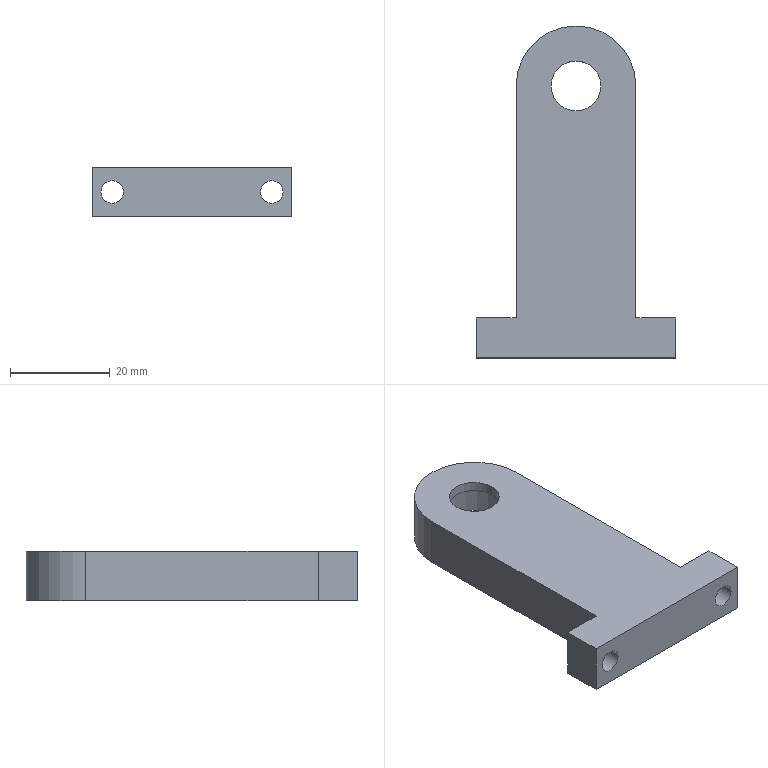Part | Creo | features CURVE 4, CUT 3, DATUM PLANE 3, COORDINATE SYSTEM 1, PROTRUSION 1 | 1 solid | 22 faces | box 40 x 66.5 x 10 mm | volume 14034 mm3 | plane 11 | cylinder 11 | commonest cylinder face diameters 4.5 x4 10 x2 15.636 x2 19 x2 24 x1
STEP:
#1=CARTESIAN_POINT('',(0.,0.,0.));
#2=DIRECTION('',(0.,0.,1.));
#3=DIRECTION('',(1.,0.,0.));
#4=AXIS2_PLACEMENT_3D('',#1,#2,#3);
#5=CARTESIAN_POINT('',(12.,54.5,0.));
#6=VERTEX_POINT('',#5);
#7=CARTESIAN_POINT('',(-12.,54.5,0.));
#8=VERTEX_POINT('',#7);
#9=CARTESIAN_POINT('',(0.,54.5,0.));
#10=DIRECTION('',(0.,0.,1.));
#11=DIRECTION('',(1.,0.,0.));
#12=AXIS2_PLACEMENT_3D('',#9,#10,#11);
#13=CIRCLE('',#12,12.);
#14=EDGE_CURVE('',#6,#8,#13,.T.);
#15=ORIENTED_EDGE('',*,*,#14,.T.);
#16=CARTESIAN_POINT('',(-12.,8.,0.));
#17=VERTEX_POINT('',#16);
#18=CARTESIAN_POINT('',(-12.,54.5,0.));
#19=DIRECTION('',(0.,-1.,0.));
#20=VECTOR('',#19,46.5);
#21=LINE('',#18,#20);
#22=EDGE_CURVE('',#8,#17,#21,.T.);
#23=ORIENTED_EDGE('',*,*,#22,.T.);
#24=CARTESIAN_POINT('',(-20.,8.,0.));
#25=VERTEX_POINT('',#24);
#26=CARTESIAN_POINT('',(-12.,8.,0.));
#27=DIRECTION('',(-1.,0.,0.));
#28=VECTOR('',#27,8.);
#29=LINE('',#26,#28);
#30=EDGE_CURVE('',#17,#25,#29,.T.);
#31=ORIENTED_EDGE('',*,*,#30,.T.);
#32=CARTESIAN_POINT('',(-20.,0.,0.));
#33=VERTEX_POINT('',#32);
#34=CARTESIAN_POINT('',(-20.,8.,0.));
#35=DIRECTION('',(0.,-1.,0.));
#36=VECTOR('',#35,8.);
#37=LINE('',#34,#36);
#38=EDGE_CURVE('',#25,#33,#37,.T.);
#39=ORIENTED_EDGE('',*,*,#38,.T.);
#40=CARTESIAN_POINT('',(20.,0.,0.));
#41=VERTEX_POINT('',#40);
#42=CARTESIAN_POINT('',(-20.,0.,0.));
#43=DIRECTION('',(1.,0.,0.));
#44=VECTOR('',#43,40.);
#45=LINE('',#42,#44);
#46=EDGE_CURVE('',#33,#41,#45,.T.);
#47=ORIENTED_EDGE('',*,*,#46,.T.);
#48=CARTESIAN_POINT('',(20.,8.,0.));
#49=VERTEX_POINT('',#48);
#50=CARTESIAN_POINT('',(20.,0.,0.));
#51=DIRECTION('',(0.,1.,0.));
#52=VECTOR('',#51,8.);
#53=LINE('',#50,#52);
#54=EDGE_CURVE('',#41,#49,#53,.T.);
#55=ORIENTED_EDGE('',*,*,#54,.T.);
#56=CARTESIAN_POINT('',(12.,8.,0.));
#57=VERTEX_POINT('',#56);
#58=CARTESIAN_POINT('',(20.,8.,0.));
#59=DIRECTION('',(-1.,0.,0.));
#60=VECTOR('',#59,8.);
#61=LINE('',#58,#60);
#62=EDGE_CURVE('',#49,#57,#61,.T.);
#63=ORIENTED_EDGE('',*,*,#62,.T.);
#64=CARTESIAN_POINT('',(12.,8.,0.));
#65=DIRECTION('',(0.,1.,0.));
#66=VECTOR('',#65,46.5);
#67=LINE('',#64,#66);
#68=EDGE_CURVE('',#57,#6,#67,.T.);
#69=ORIENTED_EDGE('',*,*,#68,.T.);
#70=EDGE_LOOP('',(#15,#23,#31,#39,#47,#55,#63,#69));
#71=FACE_OUTER_BOUND('',#70,.F.);
#72=CARTESIAN_POINT('',(-9.5,54.5,0.));
#73=VERTEX_POINT('',#72);
#74=CARTESIAN_POINT('',(9.5,54.5,0.));
#75=VERTEX_POINT('',#74);
#76=CARTESIAN_POINT('',(0.,54.5,0.));
#77=DIRECTION('',(0.,0.,-1.));
#78=DIRECTION('',(-1.,0.,0.));
#79=AXIS2_PLACEMENT_3D('',#76,#77,#78);
#80=CIRCLE('',#79,9.5);
#81=EDGE_CURVE('',#73,#75,#80,.T.);
#82=ORIENTED_EDGE('',*,*,#81,.T.);
#83=CARTESIAN_POINT('',(0.,54.5,0.));
#84=DIRECTION('',(0.,0.,-1.));
#85=DIRECTION('',(1.,0.,0.));
#86=AXIS2_PLACEMENT_3D('',#83,#84,#85);
#87=CIRCLE('',#86,9.5);
#88=EDGE_CURVE('',#75,#73,#87,.T.);
#89=ORIENTED_EDGE('',*,*,#88,.T.);
#90=EDGE_LOOP('',(#82,#89));
#91=FACE_BOUND('',#90,.F.);
#92=CARTESIAN_POINT('',(0.,0.,0.));
#93=DIRECTION('',(0.,0.,1.));
#94=DIRECTION('',(1.,0.,0.));
#95=AXIS2_PLACEMENT_3D('',#92,#93,#94);
#96=PLANE('',#95);
#97=ADVANCED_FACE('',(#71,#91),#96,.F.);
#98=ORIENTED_EDGE('',*,*,#14,.F.);
#99=CARTESIAN_POINT('',(12.,54.5,10.));
#100=VERTEX_POINT('',#99);
#101=CARTESIAN_POINT('',(12.,54.5,0.));
#102=DIRECTION('',(0.,0.,1.));
#103=VECTOR('',#102,10.);
#104=LINE('',#101,#103);
#105=EDGE_CURVE('',#6,#100,#104,.T.);
#106=ORIENTED_EDGE('',*,*,#105,.T.);
#107=CARTESIAN_POINT('',(-12.,54.5,10.));
#108=VERTEX_POINT('',#107);
#109=CARTESIAN_POINT('',(0.,54.5,10.));
#110=DIRECTION('',(0.,0.,1.));
#111=DIRECTION('',(1.,0.,0.));
#112=AXIS2_PLACEMENT_3D('',#109,#110,#111);
#113=CIRCLE('',#112,12.);
#114=EDGE_CURVE('',#100,#108,#113,.T.);
#115=ORIENTED_EDGE('',*,*,#114,.T.);
#116=CARTESIAN_POINT('',(-12.,54.5,0.));
#117=DIRECTION('',(0.,0.,1.));
#118=VECTOR('',#117,10.);
#119=LINE('',#116,#118);
#120=EDGE_CURVE('',#8,#108,#119,.T.);
#121=ORIENTED_EDGE('',*,*,#120,.F.);
#122=EDGE_LOOP('',(#98,#106,#115,#121));
#123=FACE_OUTER_BOUND('',#122,.F.);
#124=CARTESIAN_POINT('',(0.,54.5,0.));
#125=DIRECTION('',(0.,0.,1.));
#126=DIRECTION('',(1.,0.,0.));
#127=AXIS2_PLACEMENT_3D('',#124,#125,#126);
#128=CYLINDRICAL_SURFACE('',#127,12.);
#129=ADVANCED_FACE('',(#123),#128,.T.);
#130=ORIENTED_EDGE('',*,*,#68,.F.);
#131=CARTESIAN_POINT('',(12.,8.,10.));
#132=VERTEX_POINT('',#131);
#133=CARTESIAN_POINT('',(12.,8.,0.));
#134=DIRECTION('',(0.,0.,1.));
#135=VECTOR('',#134,10.);
#136=LINE('',#133,#135);
#137=EDGE_CURVE('',#57,#132,#136,.T.);
#138=ORIENTED_EDGE('',*,*,#137,.T.);
#139=CARTESIAN_POINT('',(12.,8.,10.));
#140=DIRECTION('',(0.,1.,0.));
#141=VECTOR('',#140,46.5);
#142=LINE('',#139,#141);
#143=EDGE_CURVE('',#132,#100,#142,.T.);
#144=ORIENTED_EDGE('',*,*,#143,.T.);
#145=ORIENTED_EDGE('',*,*,#105,.F.);
#146=EDGE_LOOP('',(#130,#138,#144,#145));
#147=FACE_OUTER_BOUND('',#146,.F.);
#148=CARTESIAN_POINT('',(12.,8.,0.));
#149=DIRECTION('',(1.,0.,0.));
#150=DIRECTION('',(0.,1.,0.));
#151=AXIS2_PLACEMENT_3D('',#148,#149,#150);
#152=PLANE('',#151);
#153=ADVANCED_FACE('',(#147),#152,.T.);
#154=ORIENTED_EDGE('',*,*,#62,.F.);
#155=CARTESIAN_POINT('',(20.,8.,10.));
#156=VERTEX_POINT('',#155);
#157=CARTESIAN_POINT('',(20.,8.,0.));
#158=DIRECTION('',(0.,0.,1.));
#159=VECTOR('',#158,10.);
#160=LINE('',#157,#159);
#161=EDGE_CURVE('',#49,#156,#160,.T.);
#162=ORIENTED_EDGE('',*,*,#161,.T.);
#163=CARTESIAN_POINT('',(20.,8.,10.));
#164=DIRECTION('',(-1.,0.,0.));
#165=VECTOR('',#164,8.);
#166=LINE('',#163,#165);
#167=EDGE_CURVE('',#156,#132,#166,.T.);
#168=ORIENTED_EDGE('',*,*,#167,.T.);
#169=ORIENTED_EDGE('',*,*,#137,.F.);
#170=EDGE_LOOP('',(#154,#162,#168,#169));
#171=FACE_OUTER_BOUND('',#170,.F.);
#172=CARTESIAN_POINT('',(18.25,8.,5.));
#173=VERTEX_POINT('',#172);
#174=CARTESIAN_POINT('',(13.75,8.,5.));
#175=VERTEX_POINT('',#174);
#176=CARTESIAN_POINT('',(16.,8.,5.));
#177=DIRECTION('',(0.,1.,0.));
#178=DIRECTION('',(1.,0.,0.));
#179=AXIS2_PLACEMENT_3D('',#176,#177,#178);
#180=CIRCLE('',#179,2.25);
#181=EDGE_CURVE('',#173,#175,#180,.T.);
#182=ORIENTED_EDGE('',*,*,#181,.T.);
#183=CARTESIAN_POINT('',(16.,8.,5.));
#184=DIRECTION('',(0.,1.,0.));
#185=DIRECTION('',(-1.,0.,0.));
#186=AXIS2_PLACEMENT_3D('',#183,#184,#185);
#187=CIRCLE('',#186,2.25);
#188=EDGE_CURVE('',#175,#173,#187,.T.);
#189=ORIENTED_EDGE('',*,*,#188,.T.);
#190=EDGE_LOOP('',(#182,#189));
#191=FACE_BOUND('',#190,.F.);
#192=CARTESIAN_POINT('',(20.,8.,0.));
#193=DIRECTION('',(0.,1.,0.));
#194=DIRECTION('',(-1.,0.,0.));
#195=AXIS2_PLACEMENT_3D('',#192,#193,#194);
#196=PLANE('',#195);
#197=ADVANCED_FACE('',(#171,#191),#196,.T.);
#198=ORIENTED_EDGE('',*,*,#54,.F.);
#199=CARTESIAN_POINT('',(20.,0.,10.));
#200=VERTEX_POINT('',#199);
#201=CARTESIAN_POINT('',(20.,0.,0.));
#202=DIRECTION('',(0.,0.,1.));
#203=VECTOR('',#202,10.);
#204=LINE('',#201,#203);
#205=EDGE_CURVE('',#41,#200,#204,.T.);
#206=ORIENTED_EDGE('',*,*,#205,.T.);
#207=CARTESIAN_POINT('',(20.,0.,10.));
#208=DIRECTION('',(0.,1.,0.));
#209=VECTOR('',#208,8.);
#210=LINE('',#207,#209);
#211=EDGE_CURVE('',#200,#156,#210,.T.);
#212=ORIENTED_EDGE('',*,*,#211,.T.);
#213=ORIENTED_EDGE('',*,*,#161,.F.);
#214=EDGE_LOOP('',(#198,#206,#212,#213));
#215=FACE_OUTER_BOUND('',#214,.F.);
#216=CARTESIAN_POINT('',(20.,0.,0.));
#217=DIRECTION('',(1.,0.,0.));
#218=DIRECTION('',(0.,1.,0.));
#219=AXIS2_PLACEMENT_3D('',#216,#217,#218);
#220=PLANE('',#219);
#221=ADVANCED_FACE('',(#215),#220,.T.);
#222=ORIENTED_EDGE('',*,*,#46,.F.);
#223=CARTESIAN_POINT('',(-20.,0.,10.));
#224=VERTEX_POINT('',#223);
#225=CARTESIAN_POINT('',(-20.,0.,0.));
#226=DIRECTION('',(0.,0.,1.));
#227=VECTOR('',#226,10.);
#228=LINE('',#225,#227);
#229=EDGE_CURVE('',#33,#224,#228,.T.);
#230=ORIENTED_EDGE('',*,*,#229,.T.);
#231=CARTESIAN_POINT('',(-20.,0.,10.));
#232=DIRECTION('',(1.,0.,0.));
#233=VECTOR('',#232,40.);
#234=LINE('',#231,#233);
#235=EDGE_CURVE('',#224,#200,#234,.T.);
#236=ORIENTED_EDGE('',*,*,#235,.T.);
#237=ORIENTED_EDGE('',*,*,#205,.F.);
#238=EDGE_LOOP('',(#222,#230,#236,#237));
#239=FACE_OUTER_BOUND('',#238,.F.);
#240=CARTESIAN_POINT('',(18.25,0.,5.));
#241=VERTEX_POINT('',#240);
#242=CARTESIAN_POINT('',(13.75,0.,5.));
#243=VERTEX_POINT('',#242);
#244=CARTESIAN_POINT('',(16.,0.,5.));
#245=DIRECTION('',(0.,1.,0.));
#246=DIRECTION('',(1.,0.,0.));
#247=AXIS2_PLACEMENT_3D('',#244,#245,#246);
#248=CIRCLE('',#247,2.25);
#249=EDGE_CURVE('',#241,#243,#248,.T.);
#250=ORIENTED_EDGE('',*,*,#249,.F.);
#251=CARTESIAN_POINT('',(16.,0.,5.));
#252=DIRECTION('',(0.,1.,0.));
#253=DIRECTION('',(-1.,0.,0.));
#254=AXIS2_PLACEMENT_3D('',#251,#252,#253);
#255=CIRCLE('',#254,2.25);
#256=EDGE_CURVE('',#243,#241,#255,.T.);
#257=ORIENTED_EDGE('',*,*,#256,.F.);
#258=EDGE_LOOP('',(#250,#257));
#259=FACE_BOUND('',#258,.F.);
#260=CARTESIAN_POINT('',(-13.75,0.,5.));
#261=VERTEX_POINT('',#260);
#262=CARTESIAN_POINT('',(-18.25,0.,5.));
#263=VERTEX_POINT('',#262);
#264=CARTESIAN_POINT('',(-16.,0.,5.));
#265=DIRECTION('',(0.,1.,0.));
#266=DIRECTION('',(1.,0.,0.));
#267=AXIS2_PLACEMENT_3D('',#264,#265,#266);
#268=CIRCLE('',#267,2.25);
#269=EDGE_CURVE('',#261,#263,#268,.T.);
#270=ORIENTED_EDGE('',*,*,#269,.F.);
#271=CARTESIAN_POINT('',(-16.,0.,5.));
#272=DIRECTION('',(0.,1.,0.));
#273=DIRECTION('',(-1.,0.,0.));
#274=AXIS2_PLACEMENT_3D('',#271,#272,#273);
#275=CIRCLE('',#274,2.25);
#276=EDGE_CURVE('',#263,#261,#275,.T.);
#277=ORIENTED_EDGE('',*,*,#276,.F.);
#278=EDGE_LOOP('',(#270,#277));
#279=FACE_BOUND('',#278,.F.);
#280=CARTESIAN_POINT('',(-20.,0.,0.));
#281=DIRECTION('',(0.,-1.,0.));
#282=DIRECTION('',(1.,0.,0.));
#283=AXIS2_PLACEMENT_3D('',#280,#281,#282);
#284=PLANE('',#283);
#285=ADVANCED_FACE('',(#239,#259,#279),#284,.T.);
#286=ORIENTED_EDGE('',*,*,#38,.F.);
#287=CARTESIAN_POINT('',(-20.,8.,10.));
#288=VERTEX_POINT('',#287);
#289=CARTESIAN_POINT('',(-20.,8.,0.));
#290=DIRECTION('',(0.,0.,1.));
#291=VECTOR('',#290,10.);
#292=LINE('',#289,#291);
#293=EDGE_CURVE('',#25,#288,#292,.T.);
#294=ORIENTED_EDGE('',*,*,#293,.T.);
#295=CARTESIAN_POINT('',(-20.,8.,10.));
#296=DIRECTION('',(0.,-1.,0.));
#297=VECTOR('',#296,8.);
#298=LINE('',#295,#297);
#299=EDGE_CURVE('',#288,#224,#298,.T.);
#300=ORIENTED_EDGE('',*,*,#299,.T.);
#301=ORIENTED_EDGE('',*,*,#229,.F.);
#302=EDGE_LOOP('',(#286,#294,#300,#301));
#303=FACE_OUTER_BOUND('',#302,.F.);
#304=CARTESIAN_POINT('',(-20.,8.,0.));
#305=DIRECTION('',(-1.,0.,0.));
#306=DIRECTION('',(0.,-1.,0.));
#307=AXIS2_PLACEMENT_3D('',#304,#305,#306);
#308=PLANE('',#307);
#309=ADVANCED_FACE('',(#303),#308,.T.);
#310=ORIENTED_EDGE('',*,*,#30,.F.);
#311=CARTESIAN_POINT('',(-12.,8.,10.));
#312=VERTEX_POINT('',#311);
#313=CARTESIAN_POINT('',(-12.,8.,0.));
#314=DIRECTION('',(0.,0.,1.));
#315=VECTOR('',#314,10.);
#316=LINE('',#313,#315);
#317=EDGE_CURVE('',#17,#312,#316,.T.);
#318=ORIENTED_EDGE('',*,*,#317,.T.);
#319=CARTESIAN_POINT('',(-12.,8.,10.));
#320=DIRECTION('',(-1.,0.,0.));
#321=VECTOR('',#320,8.);
#322=LINE('',#319,#321);
#323=EDGE_CURVE('',#312,#288,#322,.T.);
#324=ORIENTED_EDGE('',*,*,#323,.T.);
#325=ORIENTED_EDGE('',*,*,#293,.F.);
#326=EDGE_LOOP('',(#310,#318,#324,#325));
#327=FACE_OUTER_BOUND('',#326,.F.);
#328=CARTESIAN_POINT('',(-13.75,8.,5.));
#329=VERTEX_POINT('',#328);
#330=CARTESIAN_POINT('',(-18.25,8.,5.));
#331=VERTEX_POINT('',#330);
#332=CARTESIAN_POINT('',(-16.,8.,5.));
#333=DIRECTION('',(0.,1.,0.));
#334=DIRECTION('',(1.,0.,0.));
#335=AXIS2_PLACEMENT_3D('',#332,#333,#334);
#336=CIRCLE('',#335,2.25);
#337=EDGE_CURVE('',#329,#331,#336,.T.);
#338=ORIENTED_EDGE('',*,*,#337,.T.);
#339=CARTESIAN_POINT('',(-16.,8.,5.));
#340=DIRECTION('',(0.,1.,0.));
#341=DIRECTION('',(-1.,0.,0.));
#342=AXIS2_PLACEMENT_3D('',#339,#340,#341);
#343=CIRCLE('',#342,2.25);
#344=EDGE_CURVE('',#331,#329,#343,.T.);
#345=ORIENTED_EDGE('',*,*,#344,.T.);
#346=EDGE_LOOP('',(#338,#345));
#347=FACE_BOUND('',#346,.F.);
#348=CARTESIAN_POINT('',(-12.,8.,0.));
#349=DIRECTION('',(0.,1.,0.));
#350=DIRECTION('',(-1.,0.,0.));
#351=AXIS2_PLACEMENT_3D('',#348,#349,#350);
#352=PLANE('',#351);
#353=ADVANCED_FACE('',(#327,#347),#352,.T.);
#354=ORIENTED_EDGE('',*,*,#22,.F.);
#355=ORIENTED_EDGE('',*,*,#120,.T.);
#356=CARTESIAN_POINT('',(-12.,54.5,10.));
#357=DIRECTION('',(0.,-1.,0.));
#358=VECTOR('',#357,46.5);
#359=LINE('',#356,#358);
#360=EDGE_CURVE('',#108,#312,#359,.T.);
#361=ORIENTED_EDGE('',*,*,#360,.T.);
#362=ORIENTED_EDGE('',*,*,#317,.F.);
#363=EDGE_LOOP('',(#354,#355,#361,#362));
#364=FACE_OUTER_BOUND('',#363,.F.);
#365=CARTESIAN_POINT('',(-12.,54.5,0.));
#366=DIRECTION('',(-1.,0.,0.));
#367=DIRECTION('',(0.,-1.,0.));
#368=AXIS2_PLACEMENT_3D('',#365,#366,#367);
#369=PLANE('',#368);
#370=ADVANCED_FACE('',(#364),#369,.T.);
#371=ORIENTED_EDGE('',*,*,#114,.F.);
#372=ORIENTED_EDGE('',*,*,#143,.F.);
#373=ORIENTED_EDGE('',*,*,#167,.F.);
#374=ORIENTED_EDGE('',*,*,#211,.F.);
#375=ORIENTED_EDGE('',*,*,#235,.F.);
#376=ORIENTED_EDGE('',*,*,#299,.F.);
#377=ORIENTED_EDGE('',*,*,#323,.F.);
#378=ORIENTED_EDGE('',*,*,#360,.F.);
#379=EDGE_LOOP('',(#371,#372,#373,#374,#375,#376,#377,#378));
#380=FACE_OUTER_BOUND('',#379,.F.);
#381=CARTESIAN_POINT('',(5.,54.5,10.));
#382=VERTEX_POINT('',#381);
#383=CARTESIAN_POINT('',(-5.,54.5,10.));
#384=VERTEX_POINT('',#383);
#385=CARTESIAN_POINT('',(0.,54.5,10.));
#386=DIRECTION('',(0.,0.,-1.));
#387=DIRECTION('',(1.,0.,0.));
#388=AXIS2_PLACEMENT_3D('',#385,#386,#387);
#389=CIRCLE('',#388,5.);
#390=EDGE_CURVE('',#382,#384,#389,.T.);
#391=ORIENTED_EDGE('',*,*,#390,.F.);
#392=CARTESIAN_POINT('',(0.,54.5,10.));
#393=DIRECTION('',(0.,0.,-1.));
#394=DIRECTION('',(-1.,0.,0.));
#395=AXIS2_PLACEMENT_3D('',#392,#393,#394);
#396=CIRCLE('',#395,5.);
#397=EDGE_CURVE('',#384,#382,#396,.T.);
#398=ORIENTED_EDGE('',*,*,#397,.F.);
#399=EDGE_LOOP('',(#391,#398));
#400=FACE_BOUND('',#399,.F.);
#401=CARTESIAN_POINT('',(0.,0.,10.));
#402=DIRECTION('',(0.,0.,1.));
#403=DIRECTION('',(1.,0.,0.));
#404=AXIS2_PLACEMENT_3D('',#401,#402,#403);
#405=PLANE('',#404);
#406=ADVANCED_FACE('',(#380,#400),#405,.T.);
#407=CARTESIAN_POINT('',(-5.,54.5,8.));
#408=VERTEX_POINT('',#407);
#409=CARTESIAN_POINT('',(5.,54.5,8.));
#410=VERTEX_POINT('',#409);
#411=CARTESIAN_POINT('',(0.,54.5,8.));
#412=DIRECTION('',(0.,0.,1.));
#413=DIRECTION('',(-1.,0.,0.));
#414=AXIS2_PLACEMENT_3D('',#411,#412,#413);
#415=CIRCLE('',#414,5.);
#416=EDGE_CURVE('',#408,#410,#415,.T.);
#417=ORIENTED_EDGE('',*,*,#416,.T.);
#418=CARTESIAN_POINT('',(5.,54.5,8.));
#419=DIRECTION('',(0.,0.,1.));
#420=VECTOR('',#419,2.);
#421=LINE('',#418,#420);
#422=EDGE_CURVE('',#410,#382,#421,.T.);
#423=ORIENTED_EDGE('',*,*,#422,.T.);
#424=ORIENTED_EDGE('',*,*,#390,.T.);
#425=CARTESIAN_POINT('',(-5.,54.5,8.));
#426=DIRECTION('',(0.,0.,1.));
#427=VECTOR('',#426,2.);
#428=LINE('',#425,#427);
#429=EDGE_CURVE('',#408,#384,#428,.T.);
#430=ORIENTED_EDGE('',*,*,#429,.F.);
#431=EDGE_LOOP('',(#417,#423,#424,#430));
#432=FACE_OUTER_BOUND('',#431,.F.);
#433=CARTESIAN_POINT('',(0.,54.5,0.));
#434=DIRECTION('',(0.,0.,1.));
#435=DIRECTION('',(1.,0.,0.));
#436=AXIS2_PLACEMENT_3D('',#433,#434,#435);
#437=CYLINDRICAL_SURFACE('',#436,5.);
#438=ADVANCED_FACE('',(#432),#437,.F.);
#439=CARTESIAN_POINT('',(-7.818,54.5,8.));
#440=VERTEX_POINT('',#439);
#441=CARTESIAN_POINT('',(7.818,54.5,8.));
#442=VERTEX_POINT('',#441);
#443=CARTESIAN_POINT('',(0.,54.5,8.));
#444=DIRECTION('',(0.,0.,-1.));
#445=DIRECTION('',(-1.,0.,0.));
#446=AXIS2_PLACEMENT_3D('',#443,#444,#445);
#447=CIRCLE('',#446,7.818);
#448=EDGE_CURVE('',#440,#442,#447,.T.);
#449=ORIENTED_EDGE('',*,*,#448,.F.);
#450=CARTESIAN_POINT('',(0.,54.5,8.));
#451=DIRECTION('',(0.,0.,-1.));
#452=DIRECTION('',(1.,0.,0.));
#453=AXIS2_PLACEMENT_3D('',#450,#451,#452);
#454=CIRCLE('',#453,7.818);
#455=EDGE_CURVE('',#442,#440,#454,.T.);
#456=ORIENTED_EDGE('',*,*,#455,.F.);
#457=EDGE_LOOP('',(#449,#456));
#458=FACE_OUTER_BOUND('',#457,.F.);
#459=ORIENTED_EDGE('',*,*,#416,.F.);
#460=CARTESIAN_POINT('',(0.,54.5,8.));
#461=DIRECTION('',(0.,0.,1.));
#462=DIRECTION('',(1.,0.,0.));
#463=AXIS2_PLACEMENT_3D('',#460,#461,#462);
#464=CIRCLE('',#463,5.);
#465=EDGE_CURVE('',#410,#408,#464,.T.);
#466=ORIENTED_EDGE('',*,*,#465,.F.);
#467=EDGE_LOOP('',(#459,#466));
#468=FACE_BOUND('',#467,.F.);
#469=CARTESIAN_POINT('',(0.,0.,8.));
#470=DIRECTION('',(0.,0.,-1.));
#471=DIRECTION('',(-1.,0.,0.));
#472=AXIS2_PLACEMENT_3D('',#469,#470,#471);
#473=PLANE('',#472);
#474=ADVANCED_FACE('',(#458,#468),#473,.T.);
#475=CARTESIAN_POINT('',(-7.818,54.5,7.));
#476=VERTEX_POINT('',#475);
#477=CARTESIAN_POINT('',(7.818,54.5,7.));
#478=VERTEX_POINT('',#477);
#479=CARTESIAN_POINT('',(0.,54.5,7.));
#480=DIRECTION('',(0.,0.,-1.));
#481=DIRECTION('',(-1.,0.,0.));
#482=AXIS2_PLACEMENT_3D('',#479,#480,#481);
#483=CIRCLE('',#482,7.818);
#484=EDGE_CURVE('',#476,#478,#483,.T.);
#485=ORIENTED_EDGE('',*,*,#484,.F.);
#486=CARTESIAN_POINT('',(-7.818,54.5,7.));
#487=DIRECTION('',(0.,0.,1.));
#488=VECTOR('',#487,1.);
#489=LINE('',#486,#488);
#490=EDGE_CURVE('',#476,#440,#489,.T.);
#491=ORIENTED_EDGE('',*,*,#490,.T.);
#492=ORIENTED_EDGE('',*,*,#448,.T.);
#493=CARTESIAN_POINT('',(7.818,54.5,7.));
#494=DIRECTION('',(0.,0.,1.));
#495=VECTOR('',#494,1.);
#496=LINE('',#493,#495);
#497=EDGE_CURVE('',#478,#442,#496,.T.);
#498=ORIENTED_EDGE('',*,*,#497,.F.);
#499=EDGE_LOOP('',(#485,#491,#492,#498));
#500=FACE_OUTER_BOUND('',#499,.F.);
#501=CARTESIAN_POINT('',(0.,54.5,7.));
#502=DIRECTION('',(0.,0.,-1.));
#503=DIRECTION('',(-1.,0.,0.));
#504=AXIS2_PLACEMENT_3D('',#501,#502,#503);
#505=CYLINDRICAL_SURFACE('',#504,7.818);
#506=ADVANCED_FACE('',(#500),#505,.F.);
#507=CARTESIAN_POINT('',(-9.5,54.5,7.));
#508=VERTEX_POINT('',#507);
#509=CARTESIAN_POINT('',(9.5,54.5,7.));
#510=VERTEX_POINT('',#509);
#511=CARTESIAN_POINT('',(0.,54.5,7.));
#512=DIRECTION('',(0.,0.,-1.));
#513=DIRECTION('',(-1.,0.,0.));
#514=AXIS2_PLACEMENT_3D('',#511,#512,#513);
#515=CIRCLE('',#514,9.5);
#516=EDGE_CURVE('',#508,#510,#515,.T.);
#517=ORIENTED_EDGE('',*,*,#516,.F.);
#518=CARTESIAN_POINT('',(0.,54.5,7.));
#519=DIRECTION('',(0.,0.,-1.));
#520=DIRECTION('',(1.,0.,0.));
#521=AXIS2_PLACEMENT_3D('',#518,#519,#520);
#522=CIRCLE('',#521,9.5);
#523=EDGE_CURVE('',#510,#508,#522,.T.);
#524=ORIENTED_EDGE('',*,*,#523,.F.);
#525=EDGE_LOOP('',(#517,#524));
#526=FACE_OUTER_BOUND('',#525,.F.);
#527=ORIENTED_EDGE('',*,*,#484,.T.);
#528=CARTESIAN_POINT('',(0.,54.5,7.));
#529=DIRECTION('',(0.,0.,-1.));
#530=DIRECTION('',(1.,0.,0.));
#531=AXIS2_PLACEMENT_3D('',#528,#529,#530);
#532=CIRCLE('',#531,7.818);
#533=EDGE_CURVE('',#478,#476,#532,.T.);
#534=ORIENTED_EDGE('',*,*,#533,.T.);
#535=EDGE_LOOP('',(#527,#534));
#536=FACE_BOUND('',#535,.F.);
#537=CARTESIAN_POINT('',(0.,0.,7.));
#538=DIRECTION('',(0.,0.,-1.));
#539=DIRECTION('',(-1.,0.,0.));
#540=AXIS2_PLACEMENT_3D('',#537,#538,#539);
#541=PLANE('',#540);
#542=ADVANCED_FACE('',(#526,#536),#541,.T.);
#543=ORIENTED_EDGE('',*,*,#81,.F.);
#544=CARTESIAN_POINT('',(-9.5,54.5,0.));
#545=DIRECTION('',(0.,0.,1.));
#546=VECTOR('',#545,7.);
#547=LINE('',#544,#546);
#548=EDGE_CURVE('',#73,#508,#547,.T.);
#549=ORIENTED_EDGE('',*,*,#548,.T.);
#550=ORIENTED_EDGE('',*,*,#516,.T.);
#551=CARTESIAN_POINT('',(9.5,54.5,0.));
#552=DIRECTION('',(0.,0.,1.));
#553=VECTOR('',#552,7.);
#554=LINE('',#551,#553);
#555=EDGE_CURVE('',#75,#510,#554,.T.);
#556=ORIENTED_EDGE('',*,*,#555,.F.);
#557=EDGE_LOOP('',(#543,#549,#550,#556));
#558=FACE_OUTER_BOUND('',#557,.F.);
#559=CARTESIAN_POINT('',(0.,54.5,0.));
#560=DIRECTION('',(0.,0.,-1.));
#561=DIRECTION('',(-1.,0.,0.));
#562=AXIS2_PLACEMENT_3D('',#559,#560,#561);
#563=CYLINDRICAL_SURFACE('',#562,9.5);
#564=ADVANCED_FACE('',(#558),#563,.F.);
#565=ORIENTED_EDGE('',*,*,#88,.F.);
#566=ORIENTED_EDGE('',*,*,#555,.T.);
#567=ORIENTED_EDGE('',*,*,#523,.T.);
#568=ORIENTED_EDGE('',*,*,#548,.F.);
#569=EDGE_LOOP('',(#565,#566,#567,#568));
#570=FACE_OUTER_BOUND('',#569,.F.);
#571=CARTESIAN_POINT('',(0.,54.5,0.));
#572=DIRECTION('',(0.,0.,-1.));
#573=DIRECTION('',(-1.,0.,0.));
#574=AXIS2_PLACEMENT_3D('',#571,#572,#573);
#575=CYLINDRICAL_SURFACE('',#574,9.5);
#576=ADVANCED_FACE('',(#570),#575,.F.);
#577=ORIENTED_EDGE('',*,*,#533,.F.);
#578=ORIENTED_EDGE('',*,*,#497,.T.);
#579=ORIENTED_EDGE('',*,*,#455,.T.);
#580=ORIENTED_EDGE('',*,*,#490,.F.);
#581=EDGE_LOOP('',(#577,#578,#579,#580));
#582=FACE_OUTER_BOUND('',#581,.F.);
#583=CARTESIAN_POINT('',(0.,54.5,7.));
#584=DIRECTION('',(0.,0.,-1.));
#585=DIRECTION('',(-1.,0.,0.));
#586=AXIS2_PLACEMENT_3D('',#583,#584,#585);
#587=CYLINDRICAL_SURFACE('',#586,7.818);
#588=ADVANCED_FACE('',(#582),#587,.F.);
#589=ORIENTED_EDGE('',*,*,#465,.T.);
#590=ORIENTED_EDGE('',*,*,#429,.T.);
#591=ORIENTED_EDGE('',*,*,#397,.T.);
#592=ORIENTED_EDGE('',*,*,#422,.F.);
#593=EDGE_LOOP('',(#589,#590,#591,#592));
#594=FACE_OUTER_BOUND('',#593,.F.);
#595=CARTESIAN_POINT('',(0.,54.5,0.));
#596=DIRECTION('',(0.,0.,1.));
#597=DIRECTION('',(1.,0.,0.));
#598=AXIS2_PLACEMENT_3D('',#595,#596,#597);
#599=CYLINDRICAL_SURFACE('',#598,5.);
#600=ADVANCED_FACE('',(#594),#599,.F.);
#601=ORIENTED_EDGE('',*,*,#337,.F.);
#602=CARTESIAN_POINT('',(-13.75,8.,5.));
#603=DIRECTION('',(0.,-1.,0.));
#604=VECTOR('',#603,8.);
#605=LINE('',#602,#604);
#606=EDGE_CURVE('',#329,#261,#605,.T.);
#607=ORIENTED_EDGE('',*,*,#606,.T.);
#608=ORIENTED_EDGE('',*,*,#269,.T.);
#609=CARTESIAN_POINT('',(-18.25,8.,5.));
#610=DIRECTION('',(0.,-1.,0.));
#611=VECTOR('',#610,8.);
#612=LINE('',#609,#611);
#613=EDGE_CURVE('',#331,#263,#612,.T.);
#614=ORIENTED_EDGE('',*,*,#613,.F.);
#615=EDGE_LOOP('',(#601,#607,#608,#614));
#616=FACE_OUTER_BOUND('',#615,.F.);
#617=CARTESIAN_POINT('',(-16.,8.,5.));
#618=DIRECTION('',(0.,1.,0.));
#619=DIRECTION('',(1.,0.,0.));
#620=AXIS2_PLACEMENT_3D('',#617,#618,#619);
#621=CYLINDRICAL_SURFACE('',#620,2.25);
#622=ADVANCED_FACE('',(#616),#621,.F.);
#623=ORIENTED_EDGE('',*,*,#344,.F.);
#624=ORIENTED_EDGE('',*,*,#613,.T.);
#625=ORIENTED_EDGE('',*,*,#276,.T.);
#626=ORIENTED_EDGE('',*,*,#606,.F.);
#627=EDGE_LOOP('',(#623,#624,#625,#626));
#628=FACE_OUTER_BOUND('',#627,.F.);
#629=CARTESIAN_POINT('',(-16.,8.,5.));
#630=DIRECTION('',(0.,1.,0.));
#631=DIRECTION('',(1.,0.,0.));
#632=AXIS2_PLACEMENT_3D('',#629,#630,#631);
#633=CYLINDRICAL_SURFACE('',#632,2.25);
#634=ADVANCED_FACE('',(#628),#633,.F.);
#635=ORIENTED_EDGE('',*,*,#249,.T.);
#636=CARTESIAN_POINT('',(13.75,8.,5.));
#637=DIRECTION('',(0.,-1.,0.));
#638=VECTOR('',#637,8.);
#639=LINE('',#636,#638);
#640=EDGE_CURVE('',#175,#243,#639,.T.);
#641=ORIENTED_EDGE('',*,*,#640,.F.);
#642=ORIENTED_EDGE('',*,*,#181,.F.);
#643=CARTESIAN_POINT('',(18.25,8.,5.));
#644=DIRECTION('',(0.,-1.,0.));
#645=VECTOR('',#644,8.);
#646=LINE('',#643,#645);
#647=EDGE_CURVE('',#173,#241,#646,.T.);
#648=ORIENTED_EDGE('',*,*,#647,.T.);
#649=EDGE_LOOP('',(#635,#641,#642,#648));
#650=FACE_OUTER_BOUND('',#649,.F.);
#651=CARTESIAN_POINT('',(16.,8.,5.));
#652=DIRECTION('',(0.,1.,0.));
#653=DIRECTION('',(1.,0.,0.));
#654=AXIS2_PLACEMENT_3D('',#651,#652,#653);
#655=CYLINDRICAL_SURFACE('',#654,2.25);
#656=ADVANCED_FACE('',(#650),#655,.F.);
#657=ORIENTED_EDGE('',*,*,#256,.T.);
#658=ORIENTED_EDGE('',*,*,#647,.F.);
#659=ORIENTED_EDGE('',*,*,#188,.F.);
#660=ORIENTED_EDGE('',*,*,#640,.T.);
#661=EDGE_LOOP('',(#657,#658,#659,#660));
#662=FACE_OUTER_BOUND('',#661,.F.);
#663=CARTESIAN_POINT('',(16.,8.,5.));
#664=DIRECTION('',(0.,1.,0.));
#665=DIRECTION('',(1.,0.,0.));
#666=AXIS2_PLACEMENT_3D('',#663,#664,#665);
#667=CYLINDRICAL_SURFACE('',#666,2.25);
#668=ADVANCED_FACE('',(#662),#667,.F.);
#669=CLOSED_SHELL('',(#97,#129,#153,#197,#221,#285,#309,#353,#370,#406,#438,#474,#506,#542,#564,#576,#588,#600,#622,#634,#656,#668));
#670=MANIFOLD_SOLID_BREP('',#669);
#671=(LENGTH_UNIT()NAMED_UNIT(*)SI_UNIT(.MILLI.,.METRE.));
#672=UNCERTAINTY_MEASURE_WITH_UNIT(LENGTH_MEASURE(0.007825),#671,'','');
#673=(NAMED_UNIT(*)PLANE_ANGLE_UNIT()SI_UNIT($,.RADIAN.));
#674=PLANE_ANGLE_MEASURE_WITH_UNIT(PLANE_ANGLE_MEASURE(0.01745),#673);
#675=(CONVERSION_BASED_UNIT('DEGREE',#674)NAMED_UNIT(*)PLANE_ANGLE_UNIT());
#676=(NAMED_UNIT(*)SI_UNIT($,.STERADIAN.)SOLID_ANGLE_UNIT());
#677=(GEOMETRIC_REPRESENTATION_CONTEXT(3)GLOBAL_UNCERTAINTY_ASSIGNED_CONTEXT((#672))GLOBAL_UNIT_ASSIGNED_CONTEXT((#671,#675,#676))REPRESENTATION_CONTEXT('',''));
#678=ADVANCED_BREP_SHAPE_REPRESENTATION('',(#4,#670),#677);